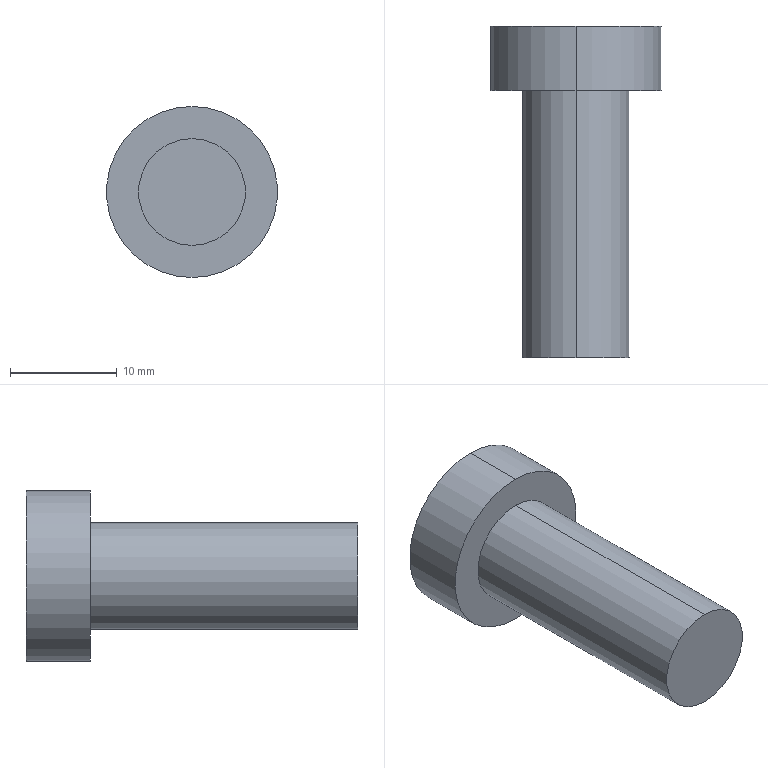Part | SolidWorks | features ICE 2, Extrusion 1 | 1 solid | 14 faces | box 16 x 31 x 16 mm | volume 2781 mm3 | plane 10 | cylinder 4 | commonest cylinder face diameters 10 x2 16 x2
STEP:
#1=CARTESIAN_POINT('',(0.,31.,8.));
#2=VERTEX_POINT('',#1);
#3=CARTESIAN_POINT('',(0.,31.,-8.));
#4=VERTEX_POINT('',#3);
#5=CARTESIAN_POINT('',(0.,31.,0.));
#6=DIRECTION('',(0.,1.,0.));
#7=DIRECTION('',(0.,0.,1.));
#8=AXIS2_PLACEMENT_3D('',#5,#6,#7);
#9=CIRCLE('',#8,8.);
#10=EDGE_CURVE('',#2,#4,#9,.T.);
#11=ORIENTED_EDGE('',*,*,#10,.F.);
#12=CARTESIAN_POINT('',(0.,25.,8.));
#13=VERTEX_POINT('',#12);
#14=CARTESIAN_POINT('',(0.,31.,8.));
#15=DIRECTION('',(0.,-1.,0.));
#16=VECTOR('',#15,1000.);
#17=LINE('',#14,#16);
#18=EDGE_CURVE('',#2,#13,#17,.T.);
#19=ORIENTED_EDGE('',*,*,#18,.T.);
#20=CARTESIAN_POINT('',(0.,25.,-8.));
#21=VERTEX_POINT('',#20);
#22=CARTESIAN_POINT('',(0.,25.,0.));
#23=DIRECTION('',(0.,1.,0.));
#24=DIRECTION('',(0.,0.,1.));
#25=AXIS2_PLACEMENT_3D('',#22,#23,#24);
#26=CIRCLE('',#25,8.);
#27=EDGE_CURVE('',#13,#21,#26,.T.);
#28=ORIENTED_EDGE('',*,*,#27,.T.);
#29=CARTESIAN_POINT('',(0.,31.,-8.));
#30=DIRECTION('',(0.,-1.,0.));
#31=VECTOR('',#30,1000.);
#32=LINE('',#29,#31);
#33=EDGE_CURVE('',#4,#21,#32,.T.);
#34=ORIENTED_EDGE('',*,*,#33,.F.);
#35=EDGE_LOOP('',(#11,#19,#28,#34));
#36=FACE_OUTER_BOUND('',#35,.T.);
#37=CARTESIAN_POINT('',(0.,31.,0.));
#38=DIRECTION('',(0.,-1.,0.));
#39=DIRECTION('',(0.,0.,-1.));
#40=AXIS2_PLACEMENT_3D('',#37,#38,#39);
#41=CYLINDRICAL_SURFACE('',#40,8.);
#42=ADVANCED_FACE('',(#36),#41,.T.);
#43=CARTESIAN_POINT('',(0.,25.,5.));
#44=VERTEX_POINT('',#43);
#45=CARTESIAN_POINT('',(0.,25.,-5.));
#46=VERTEX_POINT('',#45);
#47=CARTESIAN_POINT('',(0.,25.,0.));
#48=DIRECTION('',(0.,1.,0.));
#49=DIRECTION('',(0.,0.,1.));
#50=AXIS2_PLACEMENT_3D('',#47,#48,#49);
#51=CIRCLE('',#50,5.);
#52=EDGE_CURVE('',#44,#46,#51,.T.);
#53=ORIENTED_EDGE('',*,*,#52,.F.);
#54=CARTESIAN_POINT('',(0.,0.,5.));
#55=VERTEX_POINT('',#54);
#56=CARTESIAN_POINT('',(0.,25.,5.));
#57=DIRECTION('',(0.,-1.,0.));
#58=VECTOR('',#57,1000.);
#59=LINE('',#56,#58);
#60=EDGE_CURVE('',#44,#55,#59,.T.);
#61=ORIENTED_EDGE('',*,*,#60,.T.);
#62=CARTESIAN_POINT('',(0.,0.,-5.));
#63=VERTEX_POINT('',#62);
#64=CARTESIAN_POINT('',(0.,0.,0.));
#65=DIRECTION('',(0.,1.,0.));
#66=DIRECTION('',(0.,0.,1.));
#67=AXIS2_PLACEMENT_3D('',#64,#65,#66);
#68=CIRCLE('',#67,5.);
#69=EDGE_CURVE('',#55,#63,#68,.T.);
#70=ORIENTED_EDGE('',*,*,#69,.T.);
#71=CARTESIAN_POINT('',(0.,25.,-5.));
#72=DIRECTION('',(0.,-1.,0.));
#73=VECTOR('',#72,1000.);
#74=LINE('',#71,#73);
#75=EDGE_CURVE('',#46,#63,#74,.T.);
#76=ORIENTED_EDGE('',*,*,#75,.F.);
#77=EDGE_LOOP('',(#53,#61,#70,#76));
#78=FACE_OUTER_BOUND('',#77,.T.);
#79=CARTESIAN_POINT('',(0.,25.,0.));
#80=DIRECTION('',(0.,-1.,0.));
#81=DIRECTION('',(0.,0.,-1.));
#82=AXIS2_PLACEMENT_3D('',#79,#80,#81);
#83=CYLINDRICAL_SURFACE('',#82,5.);
#84=ADVANCED_FACE('',(#78),#83,.T.);
#85=ORIENTED_EDGE('',*,*,#60,.F.);
#86=CARTESIAN_POINT('',(0.,25.,0.));
#87=DIRECTION('',(0.,1.,0.));
#88=DIRECTION('',(0.,0.,1.));
#89=AXIS2_PLACEMENT_3D('',#86,#87,#88);
#90=CIRCLE('',#89,5.);
#91=EDGE_CURVE('',#46,#44,#90,.T.);
#92=ORIENTED_EDGE('',*,*,#91,.F.);
#93=ORIENTED_EDGE('',*,*,#75,.T.);
#94=CARTESIAN_POINT('',(0.,0.,0.));
#95=DIRECTION('',(0.,1.,0.));
#96=DIRECTION('',(0.,0.,1.));
#97=AXIS2_PLACEMENT_3D('',#94,#95,#96);
#98=CIRCLE('',#97,5.);
#99=EDGE_CURVE('',#63,#55,#98,.T.);
#100=ORIENTED_EDGE('',*,*,#99,.T.);
#101=EDGE_LOOP('',(#85,#92,#93,#100));
#102=FACE_OUTER_BOUND('',#101,.T.);
#103=CARTESIAN_POINT('',(0.,25.,0.));
#104=DIRECTION('',(0.,-1.,0.));
#105=DIRECTION('',(0.,0.,-1.));
#106=AXIS2_PLACEMENT_3D('',#103,#104,#105);
#107=CYLINDRICAL_SURFACE('',#106,5.);
#108=ADVANCED_FACE('',(#102),#107,.T.);
#109=ORIENTED_EDGE('',*,*,#99,.F.);
#110=ORIENTED_EDGE('',*,*,#69,.F.);
#111=EDGE_LOOP('',(#109,#110));
#112=FACE_OUTER_BOUND('',#111,.T.);
#113=CARTESIAN_POINT('',(0.,0.,0.));
#114=DIRECTION('',(0.,1.,0.));
#115=DIRECTION('',(0.,0.,1.));
#116=AXIS2_PLACEMENT_3D('',#113,#114,#115);
#117=PLANE('',#116);
#118=ADVANCED_FACE('',(#112),#117,.F.);
#119=ORIENTED_EDGE('',*,*,#18,.F.);
#120=CARTESIAN_POINT('',(0.,31.,0.));
#121=DIRECTION('',(0.,1.,0.));
#122=DIRECTION('',(0.,0.,1.));
#123=AXIS2_PLACEMENT_3D('',#120,#121,#122);
#124=CIRCLE('',#123,8.);
#125=EDGE_CURVE('',#4,#2,#124,.T.);
#126=ORIENTED_EDGE('',*,*,#125,.F.);
#127=ORIENTED_EDGE('',*,*,#33,.T.);
#128=CARTESIAN_POINT('',(0.,25.,0.));
#129=DIRECTION('',(0.,1.,0.));
#130=DIRECTION('',(0.,0.,1.));
#131=AXIS2_PLACEMENT_3D('',#128,#129,#130);
#132=CIRCLE('',#131,8.);
#133=EDGE_CURVE('',#21,#13,#132,.T.);
#134=ORIENTED_EDGE('',*,*,#133,.T.);
#135=EDGE_LOOP('',(#119,#126,#127,#134));
#136=FACE_OUTER_BOUND('',#135,.T.);
#137=CARTESIAN_POINT('',(0.,31.,0.));
#138=DIRECTION('',(0.,-1.,0.));
#139=DIRECTION('',(0.,0.,-1.));
#140=AXIS2_PLACEMENT_3D('',#137,#138,#139);
#141=CYLINDRICAL_SURFACE('',#140,8.);
#142=ADVANCED_FACE('',(#136),#141,.T.);
#143=CARTESIAN_POINT('',(3.826,31.,-3.912));
#144=VERTEX_POINT('',#143);
#145=CARTESIAN_POINT('',(-1.475,31.,-5.27));
#146=VERTEX_POINT('',#145);
#147=CARTESIAN_POINT('',(3.826,31.,-3.912));
#148=DIRECTION('',(-0.9687,0.,-0.2481));
#149=VECTOR('',#148,1000.);
#150=LINE('',#147,#149);
#151=EDGE_CURVE('',#144,#146,#150,.T.);
#152=ORIENTED_EDGE('',*,*,#151,.F.);
#153=CARTESIAN_POINT('',(5.301,31.,1.358));
#154=VERTEX_POINT('',#153);
#155=CARTESIAN_POINT('',(5.301,31.,1.358));
#156=DIRECTION('',(-0.2695,0.,-0.963));
#157=VECTOR('',#156,1000.);
#158=LINE('',#155,#157);
#159=EDGE_CURVE('',#154,#144,#158,.T.);
#160=ORIENTED_EDGE('',*,*,#159,.F.);
#161=CARTESIAN_POINT('',(1.475,31.,5.27));
#162=VERTEX_POINT('',#161);
#163=CARTESIAN_POINT('',(1.475,31.,5.27));
#164=DIRECTION('',(0.6992,0.,-0.7149));
#165=VECTOR('',#164,1000.);
#166=LINE('',#163,#165);
#167=EDGE_CURVE('',#162,#154,#166,.T.);
#168=ORIENTED_EDGE('',*,*,#167,.F.);
#169=CARTESIAN_POINT('',(-3.826,31.,3.912));
#170=VERTEX_POINT('',#169);
#171=CARTESIAN_POINT('',(-3.826,31.,3.912));
#172=DIRECTION('',(0.9687,0.,0.2481));
#173=VECTOR('',#172,1000.);
#174=LINE('',#171,#173);
#175=EDGE_CURVE('',#170,#162,#174,.T.);
#176=ORIENTED_EDGE('',*,*,#175,.F.);
#177=CARTESIAN_POINT('',(-5.301,31.,-1.358));
#178=VERTEX_POINT('',#177);
#179=CARTESIAN_POINT('',(-5.301,31.,-1.358));
#180=DIRECTION('',(0.2695,0.,0.963));
#181=VECTOR('',#180,1000.);
#182=LINE('',#179,#181);
#183=EDGE_CURVE('',#178,#170,#182,.T.);
#184=ORIENTED_EDGE('',*,*,#183,.F.);
#185=CARTESIAN_POINT('',(-1.475,31.,-5.27));
#186=DIRECTION('',(-0.6992,0.,0.7149));
#187=VECTOR('',#186,1000.);
#188=LINE('',#185,#187);
#189=EDGE_CURVE('',#146,#178,#188,.T.);
#190=ORIENTED_EDGE('',*,*,#189,.F.);
#191=EDGE_LOOP('',(#152,#160,#168,#176,#184,#190));
#192=FACE_BOUND('',#191,.T.);
#193=ORIENTED_EDGE('',*,*,#125,.T.);
#194=ORIENTED_EDGE('',*,*,#10,.T.);
#195=EDGE_LOOP('',(#193,#194));
#196=FACE_OUTER_BOUND('',#195,.T.);
#197=CARTESIAN_POINT('',(0.,31.,0.));
#198=DIRECTION('',(0.,1.,0.));
#199=DIRECTION('',(0.,0.,1.));
#200=AXIS2_PLACEMENT_3D('',#197,#198,#199);
#201=PLANE('',#200);
#202=ADVANCED_FACE('',(#192,#196),#201,.T.);
#203=ORIENTED_EDGE('',*,*,#91,.T.);
#204=ORIENTED_EDGE('',*,*,#52,.T.);
#205=EDGE_LOOP('',(#203,#204));
#206=FACE_BOUND('',#205,.T.);
#207=ORIENTED_EDGE('',*,*,#133,.F.);
#208=ORIENTED_EDGE('',*,*,#27,.F.);
#209=EDGE_LOOP('',(#207,#208));
#210=FACE_OUTER_BOUND('',#209,.T.);
#211=CARTESIAN_POINT('',(0.,25.,0.));
#212=DIRECTION('',(0.,1.,0.));
#213=DIRECTION('',(0.,0.,1.));
#214=AXIS2_PLACEMENT_3D('',#211,#212,#213);
#215=PLANE('',#214);
#216=ADVANCED_FACE('',(#206,#210),#215,.F.);
#217=ORIENTED_EDGE('',*,*,#151,.T.);
#218=CARTESIAN_POINT('',(-1.475,26.,-5.27));
#219=VERTEX_POINT('',#218);
#220=CARTESIAN_POINT('',(-1.475,26.,-5.27));
#221=DIRECTION('',(0.,1.,0.));
#222=VECTOR('',#221,1000.);
#223=LINE('',#220,#222);
#224=EDGE_CURVE('',#219,#146,#223,.T.);
#225=ORIENTED_EDGE('',*,*,#224,.F.);
#226=CARTESIAN_POINT('',(3.826,26.,-3.912));
#227=VERTEX_POINT('',#226);
#228=CARTESIAN_POINT('',(3.826,26.,-3.912));
#229=DIRECTION('',(-0.9687,0.,-0.2481));
#230=VECTOR('',#229,1000.);
#231=LINE('',#228,#230);
#232=EDGE_CURVE('',#227,#219,#231,.T.);
#233=ORIENTED_EDGE('',*,*,#232,.F.);
#234=CARTESIAN_POINT('',(3.826,26.,-3.912));
#235=DIRECTION('',(0.,1.,0.));
#236=VECTOR('',#235,1000.);
#237=LINE('',#234,#236);
#238=EDGE_CURVE('',#227,#144,#237,.T.);
#239=ORIENTED_EDGE('',*,*,#238,.T.);
#240=EDGE_LOOP('',(#217,#225,#233,#239));
#241=FACE_OUTER_BOUND('',#240,.T.);
#242=CARTESIAN_POINT('',(3.826,26.,-3.912));
#243=DIRECTION('',(0.2481,0.,-0.9687));
#244=DIRECTION('',(-0.9687,0.,-0.2481));
#245=AXIS2_PLACEMENT_3D('',#242,#243,#244);
#246=PLANE('',#245);
#247=ADVANCED_FACE('',(#241),#246,.F.);
#248=ORIENTED_EDGE('',*,*,#159,.T.);
#249=ORIENTED_EDGE('',*,*,#238,.F.);
#250=CARTESIAN_POINT('',(5.301,26.,1.358));
#251=VERTEX_POINT('',#250);
#252=CARTESIAN_POINT('',(5.301,26.,1.358));
#253=DIRECTION('',(-0.2695,0.,-0.963));
#254=VECTOR('',#253,1000.);
#255=LINE('',#252,#254);
#256=EDGE_CURVE('',#251,#227,#255,.T.);
#257=ORIENTED_EDGE('',*,*,#256,.F.);
#258=CARTESIAN_POINT('',(5.301,26.,1.358));
#259=DIRECTION('',(0.,1.,0.));
#260=VECTOR('',#259,1000.);
#261=LINE('',#258,#260);
#262=EDGE_CURVE('',#251,#154,#261,.T.);
#263=ORIENTED_EDGE('',*,*,#262,.T.);
#264=EDGE_LOOP('',(#248,#249,#257,#263));
#265=FACE_OUTER_BOUND('',#264,.T.);
#266=CARTESIAN_POINT('',(5.301,26.,1.358));
#267=DIRECTION('',(0.963,0.,-0.2695));
#268=DIRECTION('',(-0.2695,0.,-0.963));
#269=AXIS2_PLACEMENT_3D('',#266,#267,#268);
#270=PLANE('',#269);
#271=ADVANCED_FACE('',(#265),#270,.F.);
#272=ORIENTED_EDGE('',*,*,#167,.T.);
#273=ORIENTED_EDGE('',*,*,#262,.F.);
#274=CARTESIAN_POINT('',(1.475,26.,5.27));
#275=VERTEX_POINT('',#274);
#276=CARTESIAN_POINT('',(1.475,26.,5.27));
#277=DIRECTION('',(0.6992,0.,-0.7149));
#278=VECTOR('',#277,1000.);
#279=LINE('',#276,#278);
#280=EDGE_CURVE('',#275,#251,#279,.T.);
#281=ORIENTED_EDGE('',*,*,#280,.F.);
#282=CARTESIAN_POINT('',(1.475,26.,5.27));
#283=DIRECTION('',(0.,1.,0.));
#284=VECTOR('',#283,1000.);
#285=LINE('',#282,#284);
#286=EDGE_CURVE('',#275,#162,#285,.T.);
#287=ORIENTED_EDGE('',*,*,#286,.T.);
#288=EDGE_LOOP('',(#272,#273,#281,#287));
#289=FACE_OUTER_BOUND('',#288,.T.);
#290=CARTESIAN_POINT('',(1.475,26.,5.27));
#291=DIRECTION('',(0.7149,0.,0.6992));
#292=DIRECTION('',(0.6992,0.,-0.7149));
#293=AXIS2_PLACEMENT_3D('',#290,#291,#292);
#294=PLANE('',#293);
#295=ADVANCED_FACE('',(#289),#294,.F.);
#296=ORIENTED_EDGE('',*,*,#175,.T.);
#297=ORIENTED_EDGE('',*,*,#286,.F.);
#298=CARTESIAN_POINT('',(-3.826,26.,3.912));
#299=VERTEX_POINT('',#298);
#300=CARTESIAN_POINT('',(-3.826,26.,3.912));
#301=DIRECTION('',(0.9687,0.,0.2481));
#302=VECTOR('',#301,1000.);
#303=LINE('',#300,#302);
#304=EDGE_CURVE('',#299,#275,#303,.T.);
#305=ORIENTED_EDGE('',*,*,#304,.F.);
#306=CARTESIAN_POINT('',(-3.826,26.,3.912));
#307=DIRECTION('',(0.,1.,0.));
#308=VECTOR('',#307,1000.);
#309=LINE('',#306,#308);
#310=EDGE_CURVE('',#299,#170,#309,.T.);
#311=ORIENTED_EDGE('',*,*,#310,.T.);
#312=EDGE_LOOP('',(#296,#297,#305,#311));
#313=FACE_OUTER_BOUND('',#312,.T.);
#314=CARTESIAN_POINT('',(-3.826,26.,3.912));
#315=DIRECTION('',(-0.2481,0.,0.9687));
#316=DIRECTION('',(0.9687,0.,0.2481));
#317=AXIS2_PLACEMENT_3D('',#314,#315,#316);
#318=PLANE('',#317);
#319=ADVANCED_FACE('',(#313),#318,.F.);
#320=ORIENTED_EDGE('',*,*,#183,.T.);
#321=ORIENTED_EDGE('',*,*,#310,.F.);
#322=CARTESIAN_POINT('',(-5.301,26.,-1.358));
#323=VERTEX_POINT('',#322);
#324=CARTESIAN_POINT('',(-5.301,26.,-1.358));
#325=DIRECTION('',(0.2695,0.,0.963));
#326=VECTOR('',#325,1000.);
#327=LINE('',#324,#326);
#328=EDGE_CURVE('',#323,#299,#327,.T.);
#329=ORIENTED_EDGE('',*,*,#328,.F.);
#330=CARTESIAN_POINT('',(-5.301,26.,-1.358));
#331=DIRECTION('',(0.,1.,0.));
#332=VECTOR('',#331,1000.);
#333=LINE('',#330,#332);
#334=EDGE_CURVE('',#323,#178,#333,.T.);
#335=ORIENTED_EDGE('',*,*,#334,.T.);
#336=EDGE_LOOP('',(#320,#321,#329,#335));
#337=FACE_OUTER_BOUND('',#336,.T.);
#338=CARTESIAN_POINT('',(-5.301,26.,-1.358));
#339=DIRECTION('',(-0.963,0.,0.2695));
#340=DIRECTION('',(0.2695,0.,0.963));
#341=AXIS2_PLACEMENT_3D('',#338,#339,#340);
#342=PLANE('',#341);
#343=ADVANCED_FACE('',(#337),#342,.F.);
#344=ORIENTED_EDGE('',*,*,#189,.T.);
#345=ORIENTED_EDGE('',*,*,#334,.F.);
#346=CARTESIAN_POINT('',(-1.475,26.,-5.27));
#347=DIRECTION('',(-0.6992,0.,0.7149));
#348=VECTOR('',#347,1000.);
#349=LINE('',#346,#348);
#350=EDGE_CURVE('',#219,#323,#349,.T.);
#351=ORIENTED_EDGE('',*,*,#350,.F.);
#352=ORIENTED_EDGE('',*,*,#224,.T.);
#353=EDGE_LOOP('',(#344,#345,#351,#352));
#354=FACE_OUTER_BOUND('',#353,.T.);
#355=CARTESIAN_POINT('',(-1.475,26.,-5.27));
#356=DIRECTION('',(-0.7149,0.,-0.6992));
#357=DIRECTION('',(-0.6992,0.,0.7149));
#358=AXIS2_PLACEMENT_3D('',#355,#356,#357);
#359=PLANE('',#358);
#360=ADVANCED_FACE('',(#354),#359,.F.);
#361=ORIENTED_EDGE('',*,*,#232,.T.);
#362=ORIENTED_EDGE('',*,*,#350,.T.);
#363=ORIENTED_EDGE('',*,*,#328,.T.);
#364=ORIENTED_EDGE('',*,*,#304,.T.);
#365=ORIENTED_EDGE('',*,*,#280,.T.);
#366=ORIENTED_EDGE('',*,*,#256,.T.);
#367=EDGE_LOOP('',(#361,#362,#363,#364,#365,#366));
#368=FACE_OUTER_BOUND('',#367,.T.);
#369=CARTESIAN_POINT('',(0.,26.,0.));
#370=DIRECTION('',(0.,1.,0.));
#371=DIRECTION('',(0.,0.,1.));
#372=AXIS2_PLACEMENT_3D('',#369,#370,#371);
#373=PLANE('',#372);
#374=ADVANCED_FACE('',(#368),#373,.T.);
#375=CLOSED_SHELL('',(#42,#84,#108,#118,#142,#202,#216,#247,#271,#295,#319,#343,#360,#374));
#376=MANIFOLD_SOLID_BREP('',#375);
#377=CARTESIAN_POINT('',(0.,0.,0.));
#378=DIRECTION('',(0.,0.,1.));
#379=DIRECTION('',(1.,0.,0.));
#380=AXIS2_PLACEMENT_3D('',#377,#378,#379);
#381=(LENGTH_UNIT()NAMED_UNIT(*)SI_UNIT(.MILLI.,.METRE.));
#382=UNCERTAINTY_MEASURE_WITH_UNIT(LENGTH_MEASURE(0.00001),#381,'','');
#383=(NAMED_UNIT(*)PLANE_ANGLE_UNIT()SI_UNIT($,.RADIAN.));
#384=(NAMED_UNIT(*)SI_UNIT($,.STERADIAN.)SOLID_ANGLE_UNIT());
#385=(GEOMETRIC_REPRESENTATION_CONTEXT(3)GLOBAL_UNCERTAINTY_ASSIGNED_CONTEXT((#382))GLOBAL_UNIT_ASSIGNED_CONTEXT((#381,#383,#384))REPRESENTATION_CONTEXT('',''));
#386=ADVANCED_BREP_SHAPE_REPRESENTATION('',(#376,#380),#385);